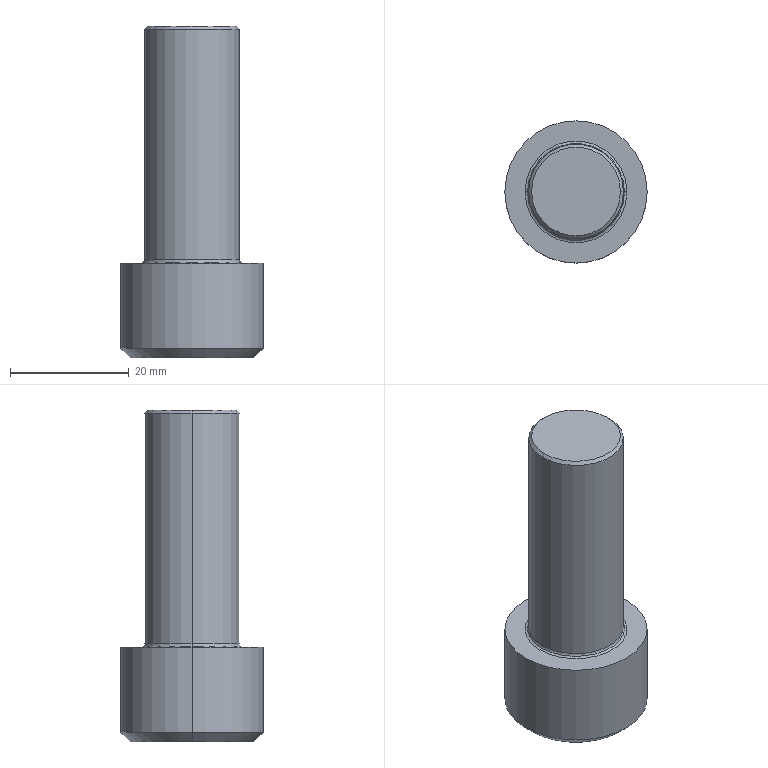Part | Creo | 1 solid | 23 faces | box 24 x 24 x 56 mm | volume 13518 mm3 | plane 9 | cone 6 | cylinder 4 | torus 4 | commonest cylinder face diameters 16 x2 24 x2
STEP:
#1=CARTESIAN_POINT('',(-223.083,-150.005,-356.));
#2=VERTEX_POINT('',#1);
#3=CARTESIAN_POINT('',(-219.041,-143.005,-356.));
#4=VERTEX_POINT('',#3);
#5=CARTESIAN_POINT('',(-223.083,-150.005,-356.));
#6=CARTESIAN_POINT('',(-222.894,-149.678,-355.891));
#7=CARTESIAN_POINT('',(-222.516,-149.023,-355.695));
#8=CARTESIAN_POINT('',(-221.94,-148.025,-355.483));
#9=CARTESIAN_POINT('',(-221.358,-147.016,-355.37));
#10=CARTESIAN_POINT('',(-220.769,-145.997,-355.37));
#11=CARTESIAN_POINT('',(-220.186,-144.986,-355.483));
#12=CARTESIAN_POINT('',(-219.61,-143.99,-355.694));
#13=CARTESIAN_POINT('',(-219.231,-143.333,-355.891));
#14=CARTESIAN_POINT('',(-219.041,-143.005,-356.));
#15=B_SPLINE_CURVE_WITH_KNOTS('',3,(#5,#6,#7,#8,#9,#10,#11,#12,#13,#14),.UNSPECIFIED.,.F.,.F.,(4,1,1,1,1,1,1,4),(0.,0.1429,0.2857,0.4286,0.5714,0.7143,0.8571,1.),.UNSPECIFIED.);
#16=EDGE_CURVE('',#2,#4,#15,.T.);
#17=ORIENTED_EDGE('',*,*,#16,.F.);
#18=CARTESIAN_POINT('',(-215.,-150.005,-351.333));
#19=VERTEX_POINT('',#18);
#20=CARTESIAN_POINT('',(-215.,-150.005,-351.333));
#21=DIRECTION('',(-0.866,0.,-0.5));
#22=VECTOR('',#21,9.333);
#23=LINE('',#20,#22);
#24=EDGE_CURVE('',#19,#2,#23,.T.);
#25=ORIENTED_EDGE('',*,*,#24,.F.);
#26=CARTESIAN_POINT('',(-206.917,-150.005,-356.));
#27=VERTEX_POINT('',#26);
#28=CARTESIAN_POINT('',(-215.,-150.005,-351.333));
#29=DIRECTION('',(0.866,0.,-0.5));
#30=VECTOR('',#29,9.333);
#31=LINE('',#28,#30);
#32=EDGE_CURVE('',#19,#27,#31,.T.);
#33=ORIENTED_EDGE('',*,*,#32,.T.);
#34=CARTESIAN_POINT('',(-210.959,-143.005,-356.));
#35=VERTEX_POINT('',#34);
#36=CARTESIAN_POINT('',(-210.959,-143.005,-356.));
#37=CARTESIAN_POINT('',(-210.77,-143.331,-355.891));
#38=CARTESIAN_POINT('',(-210.391,-143.987,-355.695));
#39=CARTESIAN_POINT('',(-209.816,-144.984,-355.483));
#40=CARTESIAN_POINT('',(-209.233,-145.993,-355.37));
#41=CARTESIAN_POINT('',(-208.644,-147.013,-355.37));
#42=CARTESIAN_POINT('',(-208.061,-148.023,-355.483));
#43=CARTESIAN_POINT('',(-207.486,-149.019,-355.694));
#44=CARTESIAN_POINT('',(-207.106,-149.677,-355.891));
#45=CARTESIAN_POINT('',(-206.917,-150.005,-356.));
#46=B_SPLINE_CURVE_WITH_KNOTS('',3,(#36,#37,#38,#39,#40,#41,#42,#43,#44,#45),.UNSPECIFIED.,.F.,.F.,(4,1,1,1,1,1,1,4),(0.,0.1429,0.2857,0.4286,0.5714,0.7143,0.8571,1.),.UNSPECIFIED.);
#47=EDGE_CURVE('',#35,#27,#46,.T.);
#48=ORIENTED_EDGE('',*,*,#47,.F.);
#49=CARTESIAN_POINT('',(-219.041,-143.005,-356.));
#50=CARTESIAN_POINT('',(-218.667,-143.005,-355.892));
#51=CARTESIAN_POINT('',(-217.914,-143.005,-355.697));
#52=CARTESIAN_POINT('',(-216.756,-143.005,-355.483));
#53=CARTESIAN_POINT('',(-215.587,-143.005,-355.37));
#54=CARTESIAN_POINT('',(-214.417,-143.005,-355.37));
#55=CARTESIAN_POINT('',(-213.25,-143.005,-355.482));
#56=CARTESIAN_POINT('',(-212.092,-143.005,-355.695));
#57=CARTESIAN_POINT('',(-211.335,-143.005,-355.891));
#58=CARTESIAN_POINT('',(-210.959,-143.005,-356.));
#59=B_SPLINE_CURVE_WITH_KNOTS('',3,(#49,#50,#51,#52,#53,#54,#55,#56,#57,#58),.UNSPECIFIED.,.F.,.F.,(4,1,1,1,1,1,1,4),(0.,0.1429,0.2857,0.4286,0.5714,0.7143,0.8571,1.),.UNSPECIFIED.);
#60=EDGE_CURVE('',#4,#35,#59,.T.);
#61=ORIENTED_EDGE('',*,*,#60,.F.);
#62=EDGE_LOOP('',(#17,#25,#33,#48,#61));
#63=FACE_OUTER_BOUND('',#62,.F.);
#64=CARTESIAN_POINT('',(-215.,-150.005,-353.713));
#65=DIRECTION('',(0.,0.,-1.));
#66=DIRECTION('',(-1.,0.,0.));
#67=AXIS2_PLACEMENT_3D('',#64,#65,#66);
#68=CONICAL_SURFACE('',#67,4.122,60.);
#69=ADVANCED_FACE('',(#63),#68,.F.);
#70=CARTESIAN_POINT('',(-219.041,-143.005,-364.));
#71=VERTEX_POINT('',#70);
#72=CARTESIAN_POINT('',(-223.083,-150.005,-364.));
#73=VERTEX_POINT('',#72);
#74=CARTESIAN_POINT('',(-219.041,-143.005,-364.));
#75=DIRECTION('',(-0.5,-0.866,0.));
#76=VECTOR('',#75,8.083);
#77=LINE('',#74,#76);
#78=EDGE_CURVE('',#71,#73,#77,.T.);
#79=ORIENTED_EDGE('',*,*,#78,.T.);
#80=CARTESIAN_POINT('',(-223.083,-150.005,-364.));
#81=DIRECTION('',(0.,0.,1.));
#82=VECTOR('',#81,8.);
#83=LINE('',#80,#82);
#84=EDGE_CURVE('',#73,#2,#83,.T.);
#85=ORIENTED_EDGE('',*,*,#84,.T.);
#86=ORIENTED_EDGE('',*,*,#16,.T.);
#87=CARTESIAN_POINT('',(-219.041,-143.005,-364.));
#88=DIRECTION('',(0.,0.,1.));
#89=VECTOR('',#88,8.);
#90=LINE('',#87,#89);
#91=EDGE_CURVE('',#71,#4,#90,.T.);
#92=ORIENTED_EDGE('',*,*,#91,.F.);
#93=EDGE_LOOP('',(#79,#85,#86,#92));
#94=FACE_OUTER_BOUND('',#93,.F.);
#95=CARTESIAN_POINT('',(-219.041,-143.005,-356.));
#96=DIRECTION('',(0.866,-0.5,0.));
#97=DIRECTION('',(-0.5,-0.866,0.));
#98=AXIS2_PLACEMENT_3D('',#95,#96,#97);
#99=PLANE('',#98);
#100=ADVANCED_FACE('',(#94),#99,.T.);
#101=CARTESIAN_POINT('',(-225.4,-150.005,-364.));
#102=VERTEX_POINT('',#101);
#103=CARTESIAN_POINT('',(-204.6,-150.005,-364.));
#104=VERTEX_POINT('',#103);
#105=CARTESIAN_POINT('',(-215.,-150.005,-364.));
#106=DIRECTION('',(0.,0.,-1.));
#107=DIRECTION('',(-1.,0.,0.));
#108=AXIS2_PLACEMENT_3D('',#105,#106,#107);
#109=CIRCLE('',#108,10.4);
#110=EDGE_CURVE('',#102,#104,#109,.T.);
#111=ORIENTED_EDGE('',*,*,#110,.F.);
#112=CARTESIAN_POINT('',(-215.,-150.005,-364.));
#113=DIRECTION('',(0.,0.,-1.));
#114=DIRECTION('',(1.,0.,0.));
#115=AXIS2_PLACEMENT_3D('',#112,#113,#114);
#116=CIRCLE('',#115,10.4);
#117=EDGE_CURVE('',#104,#102,#116,.T.);
#118=ORIENTED_EDGE('',*,*,#117,.F.);
#119=EDGE_LOOP('',(#111,#118));
#120=FACE_OUTER_BOUND('',#119,.F.);
#121=CARTESIAN_POINT('',(-219.041,-157.005,-364.));
#122=VERTEX_POINT('',#121);
#123=CARTESIAN_POINT('',(-223.083,-150.005,-364.));
#124=DIRECTION('',(0.5,-0.866,0.));
#125=VECTOR('',#124,8.083);
#126=LINE('',#123,#125);
#127=EDGE_CURVE('',#73,#122,#126,.T.);
#128=ORIENTED_EDGE('',*,*,#127,.F.);
#129=ORIENTED_EDGE('',*,*,#78,.F.);
#130=CARTESIAN_POINT('',(-210.959,-143.005,-364.));
#131=VERTEX_POINT('',#130);
#132=CARTESIAN_POINT('',(-219.041,-143.005,-364.));
#133=DIRECTION('',(1.,0.,0.));
#134=VECTOR('',#133,8.083);
#135=LINE('',#132,#134);
#136=EDGE_CURVE('',#71,#131,#135,.T.);
#137=ORIENTED_EDGE('',*,*,#136,.T.);
#138=CARTESIAN_POINT('',(-206.917,-150.005,-364.));
#139=VERTEX_POINT('',#138);
#140=CARTESIAN_POINT('',(-206.917,-150.005,-364.));
#141=DIRECTION('',(-0.5,0.866,0.));
#142=VECTOR('',#141,8.083);
#143=LINE('',#140,#142);
#144=EDGE_CURVE('',#139,#131,#143,.T.);
#145=ORIENTED_EDGE('',*,*,#144,.F.);
#146=CARTESIAN_POINT('',(-210.959,-157.005,-364.));
#147=VERTEX_POINT('',#146);
#148=CARTESIAN_POINT('',(-210.959,-157.005,-364.));
#149=DIRECTION('',(0.5,0.866,0.));
#150=VECTOR('',#149,8.083);
#151=LINE('',#148,#150);
#152=EDGE_CURVE('',#147,#139,#151,.T.);
#153=ORIENTED_EDGE('',*,*,#152,.F.);
#154=CARTESIAN_POINT('',(-210.959,-157.005,-364.));
#155=DIRECTION('',(-1.,0.,0.));
#156=VECTOR('',#155,8.083);
#157=LINE('',#154,#156);
#158=EDGE_CURVE('',#147,#122,#157,.T.);
#159=ORIENTED_EDGE('',*,*,#158,.T.);
#160=EDGE_LOOP('',(#128,#129,#137,#145,#153,#159));
#161=FACE_BOUND('',#160,.F.);
#162=CARTESIAN_POINT('',(-215.,-150.005,-364.));
#163=DIRECTION('',(0.,0.,-1.));
#164=DIRECTION('',(-1.,0.,0.));
#165=AXIS2_PLACEMENT_3D('',#162,#163,#164);
#166=PLANE('',#165);
#167=ADVANCED_FACE('',(#120,#161),#166,.T.);
#168=CARTESIAN_POINT('',(-227.,-150.005,-362.4));
#169=VERTEX_POINT('',#168);
#170=CARTESIAN_POINT('',(-203.,-150.005,-362.4));
#171=VERTEX_POINT('',#170);
#172=CARTESIAN_POINT('',(-215.,-150.005,-362.4));
#173=DIRECTION('',(0.,0.,-1.));
#174=DIRECTION('',(-1.,0.,0.));
#175=AXIS2_PLACEMENT_3D('',#172,#173,#174);
#176=CIRCLE('',#175,12.);
#177=EDGE_CURVE('',#169,#171,#176,.T.);
#178=ORIENTED_EDGE('',*,*,#177,.F.);
#179=CARTESIAN_POINT('',(-225.4,-150.005,-364.));
#180=DIRECTION('',(-0.7071,0.,0.7071));
#181=VECTOR('',#180,2.263);
#182=LINE('',#179,#181);
#183=EDGE_CURVE('',#102,#169,#182,.T.);
#184=ORIENTED_EDGE('',*,*,#183,.F.);
#185=ORIENTED_EDGE('',*,*,#110,.T.);
#186=CARTESIAN_POINT('',(-204.6,-150.005,-364.));
#187=DIRECTION('',(0.7071,0.,0.7071));
#188=VECTOR('',#187,2.263);
#189=LINE('',#186,#188);
#190=EDGE_CURVE('',#104,#171,#189,.T.);
#191=ORIENTED_EDGE('',*,*,#190,.T.);
#192=EDGE_LOOP('',(#178,#184,#185,#191));
#193=FACE_OUTER_BOUND('',#192,.F.);
#194=CARTESIAN_POINT('',(-215.,-150.005,-363.2));
#195=DIRECTION('',(0.,0.,1.));
#196=DIRECTION('',(1.,0.,0.));
#197=AXIS2_PLACEMENT_3D('',#194,#195,#196);
#198=CONICAL_SURFACE('',#197,11.2,45.);
#199=ADVANCED_FACE('',(#193),#198,.T.);
#200=ORIENTED_EDGE('',*,*,#177,.T.);
#201=CARTESIAN_POINT('',(-203.,-150.005,-348.));
#202=VERTEX_POINT('',#201);
#203=CARTESIAN_POINT('',(-203.,-150.005,-348.));
#204=DIRECTION('',(0.,0.,-1.));
#205=VECTOR('',#204,14.4);
#206=LINE('',#203,#205);
#207=EDGE_CURVE('',#202,#171,#206,.T.);
#208=ORIENTED_EDGE('',*,*,#207,.F.);
#209=CARTESIAN_POINT('',(-227.,-150.005,-348.));
#210=VERTEX_POINT('',#209);
#211=CARTESIAN_POINT('',(-215.,-150.005,-348.));
#212=DIRECTION('',(0.,0.,1.));
#213=DIRECTION('',(1.,0.,0.));
#214=AXIS2_PLACEMENT_3D('',#211,#212,#213);
#215=CIRCLE('',#214,12.);
#216=EDGE_CURVE('',#202,#210,#215,.T.);
#217=ORIENTED_EDGE('',*,*,#216,.T.);
#218=CARTESIAN_POINT('',(-227.,-150.005,-348.));
#219=DIRECTION('',(0.,0.,-1.));
#220=VECTOR('',#219,14.4);
#221=LINE('',#218,#220);
#222=EDGE_CURVE('',#210,#169,#221,.T.);
#223=ORIENTED_EDGE('',*,*,#222,.T.);
#224=EDGE_LOOP('',(#200,#208,#217,#223));
#225=FACE_OUTER_BOUND('',#224,.F.);
#226=CARTESIAN_POINT('',(-215.,-150.005,-348.));
#227=DIRECTION('',(0.,0.,-1.));
#228=DIRECTION('',(-1.,0.,0.));
#229=AXIS2_PLACEMENT_3D('',#226,#227,#228);
#230=CYLINDRICAL_SURFACE('',#229,12.);
#231=ADVANCED_FACE('',(#225),#230,.T.);
#232=CARTESIAN_POINT('',(-215.,-150.005,-362.4));
#233=DIRECTION('',(0.,0.,-1.));
#234=DIRECTION('',(1.,0.,0.));
#235=AXIS2_PLACEMENT_3D('',#232,#233,#234);
#236=CIRCLE('',#235,12.);
#237=EDGE_CURVE('',#171,#169,#236,.T.);
#238=ORIENTED_EDGE('',*,*,#237,.T.);
#239=ORIENTED_EDGE('',*,*,#222,.F.);
#240=CARTESIAN_POINT('',(-215.,-150.005,-348.));
#241=DIRECTION('',(0.,0.,1.));
#242=DIRECTION('',(-1.,0.,0.));
#243=AXIS2_PLACEMENT_3D('',#240,#241,#242);
#244=CIRCLE('',#243,12.);
#245=EDGE_CURVE('',#210,#202,#244,.T.);
#246=ORIENTED_EDGE('',*,*,#245,.T.);
#247=ORIENTED_EDGE('',*,*,#207,.T.);
#248=EDGE_LOOP('',(#238,#239,#246,#247));
#249=FACE_OUTER_BOUND('',#248,.F.);
#250=CARTESIAN_POINT('',(-215.,-150.005,-348.));
#251=DIRECTION('',(0.,0.,-1.));
#252=DIRECTION('',(-1.,0.,0.));
#253=AXIS2_PLACEMENT_3D('',#250,#251,#252);
#254=CYLINDRICAL_SURFACE('',#253,12.);
#255=ADVANCED_FACE('',(#249),#254,.T.);
#256=ORIENTED_EDGE('',*,*,#237,.F.);
#257=ORIENTED_EDGE('',*,*,#190,.F.);
#258=ORIENTED_EDGE('',*,*,#117,.T.);
#259=ORIENTED_EDGE('',*,*,#183,.T.);
#260=EDGE_LOOP('',(#256,#257,#258,#259));
#261=FACE_OUTER_BOUND('',#260,.F.);
#262=CARTESIAN_POINT('',(-215.,-150.005,-363.2));
#263=DIRECTION('',(0.,0.,1.));
#264=DIRECTION('',(1.,0.,0.));
#265=AXIS2_PLACEMENT_3D('',#262,#263,#264);
#266=CONICAL_SURFACE('',#265,11.2,45.);
#267=ADVANCED_FACE('',(#261),#266,.T.);
#268=ORIENTED_EDGE('',*,*,#245,.F.);
#269=ORIENTED_EDGE('',*,*,#216,.F.);
#270=EDGE_LOOP('',(#268,#269));
#271=FACE_OUTER_BOUND('',#270,.F.);
#272=CARTESIAN_POINT('',(-223.6,-150.005,-348.));
#273=VERTEX_POINT('',#272);
#274=CARTESIAN_POINT('',(-206.4,-150.005,-348.));
#275=VERTEX_POINT('',#274);
#276=CARTESIAN_POINT('',(-215.,-150.005,-348.));
#277=DIRECTION('',(0.,0.,-1.));
#278=DIRECTION('',(-1.,0.,0.));
#279=AXIS2_PLACEMENT_3D('',#276,#277,#278);
#280=CIRCLE('',#279,8.6);
#281=EDGE_CURVE('',#273,#275,#280,.T.);
#282=ORIENTED_EDGE('',*,*,#281,.F.);
#283=CARTESIAN_POINT('',(-215.,-150.005,-348.));
#284=DIRECTION('',(0.,0.,-1.));
#285=DIRECTION('',(1.,0.,0.));
#286=AXIS2_PLACEMENT_3D('',#283,#284,#285);
#287=CIRCLE('',#286,8.6);
#288=EDGE_CURVE('',#275,#273,#287,.T.);
#289=ORIENTED_EDGE('',*,*,#288,.F.);
#290=EDGE_LOOP('',(#282,#289));
#291=FACE_BOUND('',#290,.F.);
#292=CARTESIAN_POINT('',(-215.,-150.005,-348.));
#293=DIRECTION('',(0.,0.,-1.));
#294=DIRECTION('',(-1.,0.,0.));
#295=AXIS2_PLACEMENT_3D('',#292,#293,#294);
#296=PLANE('',#295);
#297=ADVANCED_FACE('',(#271,#291),#296,.F.);
#298=ORIENTED_EDGE('',*,*,#281,.T.);
#299=CARTESIAN_POINT('',(-206.824,-150.005,-347.824));
#300=VERTEX_POINT('',#299);
#301=CARTESIAN_POINT('',(-206.4,-150.005,-347.4));
#302=DIRECTION('',(0.,1.,0.));
#303=DIRECTION('',(0.,0.,-1.));
#304=AXIS2_PLACEMENT_3D('',#301,#302,#303);
#305=CIRCLE('',#304,0.6);
#306=EDGE_CURVE('',#275,#300,#305,.T.);
#307=ORIENTED_EDGE('',*,*,#306,.T.);
#308=CARTESIAN_POINT('',(-223.176,-150.005,-347.824));
#309=VERTEX_POINT('',#308);
#310=CARTESIAN_POINT('',(-215.,-150.005,-347.824));
#311=DIRECTION('',(0.,0.,-1.));
#312=DIRECTION('',(-1.,0.,0.));
#313=AXIS2_PLACEMENT_3D('',#310,#311,#312);
#314=CIRCLE('',#313,8.176);
#315=EDGE_CURVE('',#309,#300,#314,.T.);
#316=ORIENTED_EDGE('',*,*,#315,.F.);
#317=CARTESIAN_POINT('',(-223.6,-150.005,-347.4));
#318=DIRECTION('',(0.,-1.,0.));
#319=DIRECTION('',(0.,0.,-1.));
#320=AXIS2_PLACEMENT_3D('',#317,#318,#319);
#321=CIRCLE('',#320,0.6);
#322=EDGE_CURVE('',#273,#309,#321,.T.);
#323=ORIENTED_EDGE('',*,*,#322,.F.);
#324=EDGE_LOOP('',(#298,#307,#316,#323));
#325=FACE_OUTER_BOUND('',#324,.F.);
#326=CARTESIAN_POINT('',(-215.,-150.005,-347.4));
#327=DIRECTION('',(0.,0.,-1.));
#328=DIRECTION('',(-1.,0.,0.));
#329=AXIS2_PLACEMENT_3D('',#326,#327,#328);
#330=TOROIDAL_SURFACE('',#329,8.6,0.6);
#331=ADVANCED_FACE('',(#325),#330,.F.);
#332=ORIENTED_EDGE('',*,*,#288,.T.);
#333=ORIENTED_EDGE('',*,*,#322,.T.);
#334=CARTESIAN_POINT('',(-215.,-150.005,-347.824));
#335=DIRECTION('',(0.,0.,-1.));
#336=DIRECTION('',(1.,0.,0.));
#337=AXIS2_PLACEMENT_3D('',#334,#335,#336);
#338=CIRCLE('',#337,8.176);
#339=EDGE_CURVE('',#300,#309,#338,.T.);
#340=ORIENTED_EDGE('',*,*,#339,.F.);
#341=ORIENTED_EDGE('',*,*,#306,.F.);
#342=EDGE_LOOP('',(#332,#333,#340,#341));
#343=FACE_OUTER_BOUND('',#342,.F.);
#344=CARTESIAN_POINT('',(-215.,-150.005,-347.4));
#345=DIRECTION('',(0.,0.,-1.));
#346=DIRECTION('',(-1.,0.,0.));
#347=AXIS2_PLACEMENT_3D('',#344,#345,#346);
#348=TOROIDAL_SURFACE('',#347,8.6,0.6);
#349=ADVANCED_FACE('',(#343),#348,.F.);
#350=CARTESIAN_POINT('',(-207.,-150.005,-347.4));
#351=VERTEX_POINT('',#350);
#352=CARTESIAN_POINT('',(-223.,-150.005,-347.4));
#353=VERTEX_POINT('',#352);
#354=CARTESIAN_POINT('',(-215.,-150.005,-347.4));
#355=DIRECTION('',(0.,0.,-1.));
#356=DIRECTION('',(1.,0.,0.));
#357=AXIS2_PLACEMENT_3D('',#354,#355,#356);
#358=CIRCLE('',#357,8.);
#359=EDGE_CURVE('',#351,#353,#358,.T.);
#360=ORIENTED_EDGE('',*,*,#359,.F.);
#361=CARTESIAN_POINT('',(-206.4,-150.005,-347.4));
#362=DIRECTION('',(0.,1.,0.));
#363=DIRECTION('',(-0.7071,0.,-0.7071));
#364=AXIS2_PLACEMENT_3D('',#361,#362,#363);
#365=CIRCLE('',#364,0.6);
#366=EDGE_CURVE('',#300,#351,#365,.T.);
#367=ORIENTED_EDGE('',*,*,#366,.F.);
#368=ORIENTED_EDGE('',*,*,#339,.T.);
#369=CARTESIAN_POINT('',(-223.6,-150.005,-347.4));
#370=DIRECTION('',(0.,-1.,0.));
#371=DIRECTION('',(0.7071,0.,-0.7071));
#372=AXIS2_PLACEMENT_3D('',#369,#370,#371);
#373=CIRCLE('',#372,0.6);
#374=EDGE_CURVE('',#309,#353,#373,.T.);
#375=ORIENTED_EDGE('',*,*,#374,.T.);
#376=EDGE_LOOP('',(#360,#367,#368,#375));
#377=FACE_OUTER_BOUND('',#376,.F.);
#378=CARTESIAN_POINT('',(-215.,-150.005,-347.4));
#379=DIRECTION('',(0.,0.,-1.));
#380=DIRECTION('',(-1.,0.,0.));
#381=AXIS2_PLACEMENT_3D('',#378,#379,#380);
#382=TOROIDAL_SURFACE('',#381,8.6,0.6);
#383=ADVANCED_FACE('',(#377),#382,.F.);
#384=CARTESIAN_POINT('',(-223.,-150.005,-308.5));
#385=VERTEX_POINT('',#384);
#386=CARTESIAN_POINT('',(-207.,-150.005,-308.5));
#387=VERTEX_POINT('',#386);
#388=CARTESIAN_POINT('',(-215.,-150.005,-308.5));
#389=DIRECTION('',(0.,0.,1.));
#390=DIRECTION('',(-1.,0.,0.));
#391=AXIS2_PLACEMENT_3D('',#388,#389,#390);
#392=CIRCLE('',#391,8.);
#393=EDGE_CURVE('',#385,#387,#392,.T.);
#394=ORIENTED_EDGE('',*,*,#393,.T.);
#395=CARTESIAN_POINT('',(-207.,-150.005,-308.5));
#396=DIRECTION('',(0.,0.,-1.));
#397=VECTOR('',#396,38.9);
#398=LINE('',#395,#397);
#399=EDGE_CURVE('',#387,#351,#398,.T.);
#400=ORIENTED_EDGE('',*,*,#399,.T.);
#401=ORIENTED_EDGE('',*,*,#359,.T.);
#402=CARTESIAN_POINT('',(-223.,-150.005,-308.5));
#403=DIRECTION('',(0.,0.,-1.));
#404=VECTOR('',#403,38.9);
#405=LINE('',#402,#404);
#406=EDGE_CURVE('',#385,#353,#405,.T.);
#407=ORIENTED_EDGE('',*,*,#406,.F.);
#408=EDGE_LOOP('',(#394,#400,#401,#407));
#409=FACE_OUTER_BOUND('',#408,.F.);
#410=CARTESIAN_POINT('',(-215.,-150.005,-308.));
#411=DIRECTION('',(0.,0.,-1.));
#412=DIRECTION('',(-1.,0.,0.));
#413=AXIS2_PLACEMENT_3D('',#410,#411,#412);
#414=CYLINDRICAL_SURFACE('',#413,8.);
#415=ADVANCED_FACE('',(#409),#414,.T.);
#416=CARTESIAN_POINT('',(-222.5,-150.005,-308.));
#417=VERTEX_POINT('',#416);
#418=CARTESIAN_POINT('',(-207.5,-150.005,-308.));
#419=VERTEX_POINT('',#418);
#420=CARTESIAN_POINT('',(-215.,-150.005,-308.));
#421=DIRECTION('',(0.,0.,1.));
#422=DIRECTION('',(-1.,0.,0.));
#423=AXIS2_PLACEMENT_3D('',#420,#421,#422);
#424=CIRCLE('',#423,7.5);
#425=EDGE_CURVE('',#417,#419,#424,.T.);
#426=ORIENTED_EDGE('',*,*,#425,.T.);
#427=CARTESIAN_POINT('',(-207.5,-150.005,-308.));
#428=DIRECTION('',(0.7071,0.,-0.7071));
#429=VECTOR('',#428,0.7071);
#430=LINE('',#427,#429);
#431=EDGE_CURVE('',#419,#387,#430,.T.);
#432=ORIENTED_EDGE('',*,*,#431,.T.);
#433=ORIENTED_EDGE('',*,*,#393,.F.);
#434=CARTESIAN_POINT('',(-222.5,-150.005,-308.));
#435=DIRECTION('',(-0.7071,0.,-0.7071));
#436=VECTOR('',#435,0.7071);
#437=LINE('',#434,#436);
#438=EDGE_CURVE('',#417,#385,#437,.T.);
#439=ORIENTED_EDGE('',*,*,#438,.F.);
#440=EDGE_LOOP('',(#426,#432,#433,#439));
#441=FACE_OUTER_BOUND('',#440,.F.);
#442=CARTESIAN_POINT('',(-215.,-150.005,-308.25));
#443=DIRECTION('',(0.,0.,-1.));
#444=DIRECTION('',(-1.,0.,0.));
#445=AXIS2_PLACEMENT_3D('',#442,#443,#444);
#446=CONICAL_SURFACE('',#445,7.75,45.);
#447=ADVANCED_FACE('',(#441),#446,.T.);
#448=ORIENTED_EDGE('',*,*,#425,.F.);
#449=CARTESIAN_POINT('',(-215.,-150.005,-308.));
#450=DIRECTION('',(0.,0.,1.));
#451=DIRECTION('',(1.,0.,0.));
#452=AXIS2_PLACEMENT_3D('',#449,#450,#451);
#453=CIRCLE('',#452,7.5);
#454=EDGE_CURVE('',#419,#417,#453,.T.);
#455=ORIENTED_EDGE('',*,*,#454,.F.);
#456=EDGE_LOOP('',(#448,#455));
#457=FACE_OUTER_BOUND('',#456,.F.);
#458=CARTESIAN_POINT('',(-215.,-150.005,-308.));
#459=DIRECTION('',(0.,0.,-1.));
#460=DIRECTION('',(-1.,0.,0.));
#461=AXIS2_PLACEMENT_3D('',#458,#459,#460);
#462=PLANE('',#461);
#463=ADVANCED_FACE('',(#457),#462,.F.);
#464=ORIENTED_EDGE('',*,*,#454,.T.);
#465=ORIENTED_EDGE('',*,*,#438,.T.);
#466=CARTESIAN_POINT('',(-215.,-150.005,-308.5));
#467=DIRECTION('',(0.,0.,1.));
#468=DIRECTION('',(1.,0.,0.));
#469=AXIS2_PLACEMENT_3D('',#466,#467,#468);
#470=CIRCLE('',#469,8.);
#471=EDGE_CURVE('',#387,#385,#470,.T.);
#472=ORIENTED_EDGE('',*,*,#471,.F.);
#473=ORIENTED_EDGE('',*,*,#431,.F.);
#474=EDGE_LOOP('',(#464,#465,#472,#473));
#475=FACE_OUTER_BOUND('',#474,.F.);
#476=CARTESIAN_POINT('',(-215.,-150.005,-308.25));
#477=DIRECTION('',(0.,0.,-1.));
#478=DIRECTION('',(-1.,0.,0.));
#479=AXIS2_PLACEMENT_3D('',#476,#477,#478);
#480=CONICAL_SURFACE('',#479,7.75,45.);
#481=ADVANCED_FACE('',(#475),#480,.T.);
#482=ORIENTED_EDGE('',*,*,#471,.T.);
#483=ORIENTED_EDGE('',*,*,#406,.T.);
#484=CARTESIAN_POINT('',(-215.,-150.005,-347.4));
#485=DIRECTION('',(0.,0.,-1.));
#486=DIRECTION('',(-1.,0.,0.));
#487=AXIS2_PLACEMENT_3D('',#484,#485,#486);
#488=CIRCLE('',#487,8.);
#489=EDGE_CURVE('',#353,#351,#488,.T.);
#490=ORIENTED_EDGE('',*,*,#489,.T.);
#491=ORIENTED_EDGE('',*,*,#399,.F.);
#492=EDGE_LOOP('',(#482,#483,#490,#491));
#493=FACE_OUTER_BOUND('',#492,.F.);
#494=CARTESIAN_POINT('',(-215.,-150.005,-308.));
#495=DIRECTION('',(0.,0.,-1.));
#496=DIRECTION('',(-1.,0.,0.));
#497=AXIS2_PLACEMENT_3D('',#494,#495,#496);
#498=CYLINDRICAL_SURFACE('',#497,8.);
#499=ADVANCED_FACE('',(#493),#498,.T.);
#500=ORIENTED_EDGE('',*,*,#489,.F.);
#501=ORIENTED_EDGE('',*,*,#374,.F.);
#502=ORIENTED_EDGE('',*,*,#315,.T.);
#503=ORIENTED_EDGE('',*,*,#366,.T.);
#504=EDGE_LOOP('',(#500,#501,#502,#503));
#505=FACE_OUTER_BOUND('',#504,.F.);
#506=CARTESIAN_POINT('',(-215.,-150.005,-347.4));
#507=DIRECTION('',(0.,0.,-1.));
#508=DIRECTION('',(-1.,0.,0.));
#509=AXIS2_PLACEMENT_3D('',#506,#507,#508);
#510=TOROIDAL_SURFACE('',#509,8.6,0.6);
#511=ADVANCED_FACE('',(#505),#510,.F.);
#512=ORIENTED_EDGE('',*,*,#127,.T.);
#513=CARTESIAN_POINT('',(-219.041,-157.005,-356.));
#514=VERTEX_POINT('',#513);
#515=CARTESIAN_POINT('',(-219.041,-157.005,-364.));
#516=DIRECTION('',(0.,0.,1.));
#517=VECTOR('',#516,8.);
#518=LINE('',#515,#517);
#519=EDGE_CURVE('',#122,#514,#518,.T.);
#520=ORIENTED_EDGE('',*,*,#519,.T.);
#521=CARTESIAN_POINT('',(-219.041,-157.005,-356.));
#522=CARTESIAN_POINT('',(-219.23,-156.678,-355.891));
#523=CARTESIAN_POINT('',(-219.609,-156.023,-355.695));
#524=CARTESIAN_POINT('',(-220.184,-155.025,-355.483));
#525=CARTESIAN_POINT('',(-220.767,-154.016,-355.37));
#526=CARTESIAN_POINT('',(-221.356,-152.997,-355.37));
#527=CARTESIAN_POINT('',(-221.939,-151.986,-355.483));
#528=CARTESIAN_POINT('',(-222.514,-150.99,-355.694));
#529=CARTESIAN_POINT('',(-222.894,-150.333,-355.891));
#530=CARTESIAN_POINT('',(-223.083,-150.005,-356.));
#531=B_SPLINE_CURVE_WITH_KNOTS('',3,(#521,#522,#523,#524,#525,#526,#527,#528,#529,#530),.UNSPECIFIED.,.F.,.F.,(4,1,1,1,1,1,1,4),(0.,0.1429,0.2857,0.4286,0.5714,0.7143,0.8571,1.),.UNSPECIFIED.);
#532=EDGE_CURVE('',#514,#2,#531,.T.);
#533=ORIENTED_EDGE('',*,*,#532,.T.);
#534=ORIENTED_EDGE('',*,*,#84,.F.);
#535=EDGE_LOOP('',(#512,#520,#533,#534));
#536=FACE_OUTER_BOUND('',#535,.F.);
#537=CARTESIAN_POINT('',(-223.083,-150.005,-356.));
#538=DIRECTION('',(0.866,0.5,0.));
#539=DIRECTION('',(0.5,-0.866,0.));
#540=AXIS2_PLACEMENT_3D('',#537,#538,#539);
#541=PLANE('',#540);
#542=ADVANCED_FACE('',(#536),#541,.T.);
#543=ORIENTED_EDGE('',*,*,#158,.F.);
#544=CARTESIAN_POINT('',(-210.959,-157.005,-356.));
#545=VERTEX_POINT('',#544);
#546=CARTESIAN_POINT('',(-210.959,-157.005,-364.));
#547=DIRECTION('',(0.,0.,1.));
#548=VECTOR('',#547,8.);
#549=LINE('',#546,#548);
#550=EDGE_CURVE('',#147,#545,#549,.T.);
#551=ORIENTED_EDGE('',*,*,#550,.T.);
#552=CARTESIAN_POINT('',(-210.959,-157.005,-356.));
#553=CARTESIAN_POINT('',(-211.335,-157.005,-355.891));
#554=CARTESIAN_POINT('',(-212.092,-157.005,-355.695));
#555=CARTESIAN_POINT('',(-213.25,-157.005,-355.482));
#556=CARTESIAN_POINT('',(-214.417,-157.005,-355.37));
#557=CARTESIAN_POINT('',(-215.587,-157.005,-355.37));
#558=CARTESIAN_POINT('',(-216.756,-157.005,-355.483));
#559=CARTESIAN_POINT('',(-217.914,-157.005,-355.697));
#560=CARTESIAN_POINT('',(-218.667,-157.005,-355.892));
#561=CARTESIAN_POINT('',(-219.041,-157.005,-356.));
#562=B_SPLINE_CURVE_WITH_KNOTS('',3,(#552,#553,#554,#555,#556,#557,#558,#559,#560,#561),.UNSPECIFIED.,.F.,.F.,(4,1,1,1,1,1,1,4),(0.,0.1429,0.2857,0.4286,0.5714,0.7143,0.8571,1.),.UNSPECIFIED.);
#563=EDGE_CURVE('',#545,#514,#562,.T.);
#564=ORIENTED_EDGE('',*,*,#563,.T.);
#565=ORIENTED_EDGE('',*,*,#519,.F.);
#566=EDGE_LOOP('',(#543,#551,#564,#565));
#567=FACE_OUTER_BOUND('',#566,.F.);
#568=CARTESIAN_POINT('',(-219.041,-157.005,-356.));
#569=DIRECTION('',(0.,1.,0.));
#570=DIRECTION('',(0.,0.,-1.));
#571=AXIS2_PLACEMENT_3D('',#568,#569,#570);
#572=PLANE('',#571);
#573=ADVANCED_FACE('',(#567),#572,.T.);
#574=ORIENTED_EDGE('',*,*,#152,.T.);
#575=CARTESIAN_POINT('',(-206.917,-150.005,-364.));
#576=DIRECTION('',(0.,0.,1.));
#577=VECTOR('',#576,8.);
#578=LINE('',#575,#577);
#579=EDGE_CURVE('',#139,#27,#578,.T.);
#580=ORIENTED_EDGE('',*,*,#579,.T.);
#581=CARTESIAN_POINT('',(-206.917,-150.005,-356.));
#582=CARTESIAN_POINT('',(-207.106,-150.333,-355.891));
#583=CARTESIAN_POINT('',(-207.486,-150.99,-355.694));
#584=CARTESIAN_POINT('',(-208.061,-151.986,-355.483));
#585=CARTESIAN_POINT('',(-208.644,-152.997,-355.37));
#586=CARTESIAN_POINT('',(-209.233,-154.016,-355.37));
#587=CARTESIAN_POINT('',(-209.816,-155.025,-355.483));
#588=CARTESIAN_POINT('',(-210.391,-156.023,-355.695));
#589=CARTESIAN_POINT('',(-210.77,-156.678,-355.891));
#590=CARTESIAN_POINT('',(-210.959,-157.005,-356.));
#591=B_SPLINE_CURVE_WITH_KNOTS('',3,(#581,#582,#583,#584,#585,#586,#587,#588,#589,#590),.UNSPECIFIED.,.F.,.F.,(4,1,1,1,1,1,1,4),(0.,0.1429,0.2857,0.4286,0.5714,0.7143,0.8571,1.),.UNSPECIFIED.);
#592=EDGE_CURVE('',#27,#545,#591,.T.);
#593=ORIENTED_EDGE('',*,*,#592,.T.);
#594=ORIENTED_EDGE('',*,*,#550,.F.);
#595=EDGE_LOOP('',(#574,#580,#593,#594));
#596=FACE_OUTER_BOUND('',#595,.F.);
#597=CARTESIAN_POINT('',(-210.959,-157.005,-356.));
#598=DIRECTION('',(-0.866,0.5,0.));
#599=DIRECTION('',(0.5,0.866,0.));
#600=AXIS2_PLACEMENT_3D('',#597,#598,#599);
#601=PLANE('',#600);
#602=ADVANCED_FACE('',(#596),#601,.T.);
#603=ORIENTED_EDGE('',*,*,#144,.T.);
#604=CARTESIAN_POINT('',(-210.959,-143.005,-364.));
#605=DIRECTION('',(0.,0.,1.));
#606=VECTOR('',#605,8.);
#607=LINE('',#604,#606);
#608=EDGE_CURVE('',#131,#35,#607,.T.);
#609=ORIENTED_EDGE('',*,*,#608,.T.);
#610=ORIENTED_EDGE('',*,*,#47,.T.);
#611=ORIENTED_EDGE('',*,*,#579,.F.);
#612=EDGE_LOOP('',(#603,#609,#610,#611));
#613=FACE_OUTER_BOUND('',#612,.F.);
#614=CARTESIAN_POINT('',(-206.917,-150.005,-356.));
#615=DIRECTION('',(-0.866,-0.5,0.));
#616=DIRECTION('',(-0.5,0.866,0.));
#617=AXIS2_PLACEMENT_3D('',#614,#615,#616);
#618=PLANE('',#617);
#619=ADVANCED_FACE('',(#613),#618,.T.);
#620=ORIENTED_EDGE('',*,*,#136,.F.);
#621=ORIENTED_EDGE('',*,*,#91,.T.);
#622=ORIENTED_EDGE('',*,*,#60,.T.);
#623=ORIENTED_EDGE('',*,*,#608,.F.);
#624=EDGE_LOOP('',(#620,#621,#622,#623));
#625=FACE_OUTER_BOUND('',#624,.F.);
#626=CARTESIAN_POINT('',(-210.959,-143.005,-356.));
#627=DIRECTION('',(0.,-1.,0.));
#628=DIRECTION('',(0.,0.,1.));
#629=AXIS2_PLACEMENT_3D('',#626,#627,#628);
#630=PLANE('',#629);
#631=ADVANCED_FACE('',(#625),#630,.T.);
#632=ORIENTED_EDGE('',*,*,#592,.F.);
#633=ORIENTED_EDGE('',*,*,#32,.F.);
#634=ORIENTED_EDGE('',*,*,#24,.T.);
#635=ORIENTED_EDGE('',*,*,#532,.F.);
#636=ORIENTED_EDGE('',*,*,#563,.F.);
#637=EDGE_LOOP('',(#632,#633,#634,#635,#636));
#638=FACE_OUTER_BOUND('',#637,.F.);
#639=CARTESIAN_POINT('',(-215.,-150.005,-353.713));
#640=DIRECTION('',(0.,0.,-1.));
#641=DIRECTION('',(-1.,0.,0.));
#642=AXIS2_PLACEMENT_3D('',#639,#640,#641);
#643=CONICAL_SURFACE('',#642,4.122,60.);
#644=ADVANCED_FACE('',(#638),#643,.F.);
#645=CLOSED_SHELL('',(#69,#100,#167,#199,#231,#255,#267,#297,#331,#349,#383,#415,#447,#463,#481,#499,#511,#542,#573,#602,#619,#631,#644));
#646=MANIFOLD_SOLID_BREP('',#645);
#647=(LENGTH_UNIT()NAMED_UNIT(*)SI_UNIT(.MILLI.,.METRE.));
#648=UNCERTAINTY_MEASURE_WITH_UNIT(LENGTH_MEASURE(0.006548),#647,'','');
#649=(NAMED_UNIT(*)PLANE_ANGLE_UNIT()SI_UNIT($,.RADIAN.));
#650=PLANE_ANGLE_MEASURE_WITH_UNIT(PLANE_ANGLE_MEASURE(0.01745),#649);
#651=(CONVERSION_BASED_UNIT('DEGREE',#650)NAMED_UNIT(*)PLANE_ANGLE_UNIT());
#652=(NAMED_UNIT(*)SI_UNIT($,.STERADIAN.)SOLID_ANGLE_UNIT());
#653=(GEOMETRIC_REPRESENTATION_CONTEXT(3)GLOBAL_UNCERTAINTY_ASSIGNED_CONTEXT((#648))GLOBAL_UNIT_ASSIGNED_CONTEXT((#647,#651,#652))REPRESENTATION_CONTEXT('',''));
#654=ADVANCED_BREP_SHAPE_REPRESENTATION('',(#646),#653);